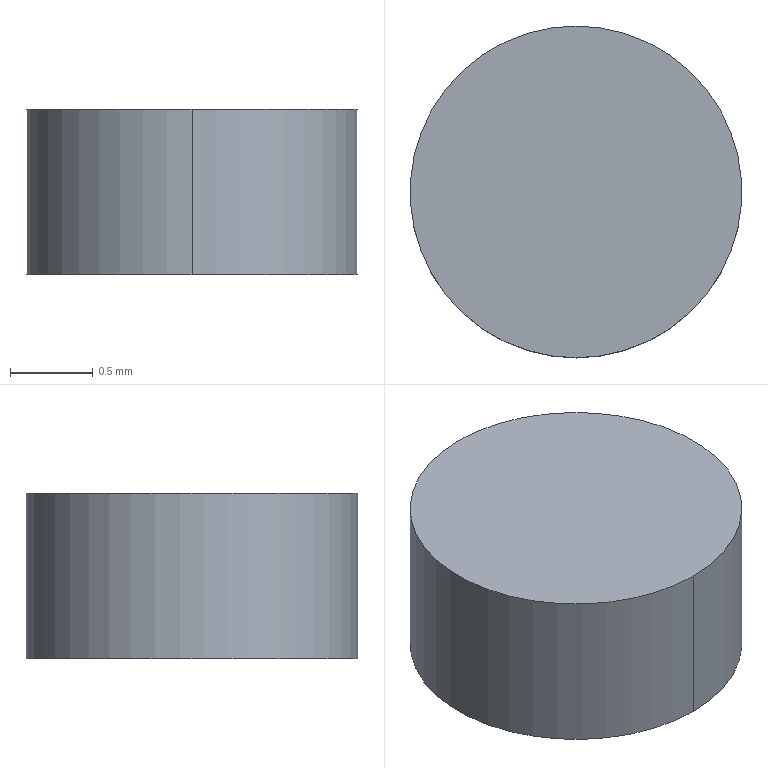Part | STEP file | 1 solid | 4 faces | box 2 x 2 x 1 mm | volume 3.142 mm3 | plane 2 | cylinder 2 | commonest cylinder face diameters 2 x2
STEP:
#1=CARTESIAN_POINT('',(0.,0.,0.));
#2=DIRECTION('',(0.,0.,1.));
#3=DIRECTION('',(1.,0.,0.));
#4=AXIS2_PLACEMENT_3D('',#1,#2,#3);
#5=CARTESIAN_POINT('',(-545.073,5728.073,1777.644));
#6=VERTEX_POINT('',#5);
#7=CARTESIAN_POINT('',(-545.073,5726.073,1777.644));
#8=VERTEX_POINT('',#7);
#9=CARTESIAN_POINT('',(-545.073,5727.073,1777.644));
#10=DIRECTION('',(0.,0.,-1.));
#11=DIRECTION('',(0.,1.,0.));
#12=AXIS2_PLACEMENT_3D('',#9,#10,#11);
#13=CIRCLE('',#12,1.);
#14=CARTESIAN_POINT('',(-529.573,5742.573,1777.644));
#15=DIRECTION('',(0.,0.,-1.));
#16=DIRECTION('',(-1.,0.,0.));
#17=AXIS2_PLACEMENT_3D('',#14,#15,#16);
#18=PLANE('',#17);
#19=CARTESIAN_POINT('',(15.5,-15.5));
#20=DIRECTION('',(0.,1.));
#21=AXIS2_PLACEMENT_2D('',#19,#20);
#22=CIRCLE('',#21,1.);
#23=(GEOMETRIC_REPRESENTATION_CONTEXT(2)PARAMETRIC_REPRESENTATION_CONTEXT()REPRESENTATION_CONTEXT('',''));
#24=DEFINITIONAL_REPRESENTATION('',(#22),#23);
#25=PCURVE('',#18,#24);
#26=CARTESIAN_POINT('',(-545.073,5727.073,1778.144));
#27=DIRECTION('',(0.,0.,1.));
#28=DIRECTION('',(0.,1.,0.));
#29=AXIS2_PLACEMENT_3D('',#26,#27,#28);
#30=CYLINDRICAL_SURFACE('',#29,1.);
#31=CARTESIAN_POINT('',(6.283,-0.5));
#32=DIRECTION('',(-1.,0.));
#33=VECTOR('',#32,1.);
#34=LINE('',#31,#33);
#35=(GEOMETRIC_REPRESENTATION_CONTEXT(2)PARAMETRIC_REPRESENTATION_CONTEXT()REPRESENTATION_CONTEXT('',''));
#36=DEFINITIONAL_REPRESENTATION('',(#34),#35);
#37=PCURVE('',#30,#36);
#38=SURFACE_CURVE('',#13,(#25,#37),.PCURVE_S1.);
#39=EDGE_CURVE('',#6,#8,#38,.T.);
#40=ORIENTED_EDGE('',*,*,#39,.F.);
#41=CARTESIAN_POINT('',(-545.073,5727.073,1777.644));
#42=DIRECTION('',(0.,0.,-1.));
#43=DIRECTION('',(0.,-1.,0.));
#44=AXIS2_PLACEMENT_3D('',#41,#42,#43);
#45=CIRCLE('',#44,1.);
#46=CARTESIAN_POINT('',(15.5,-15.5));
#47=DIRECTION('',(0.,-1.));
#48=AXIS2_PLACEMENT_2D('',#46,#47);
#49=CIRCLE('',#48,1.);
#50=(GEOMETRIC_REPRESENTATION_CONTEXT(2)PARAMETRIC_REPRESENTATION_CONTEXT()REPRESENTATION_CONTEXT('',''));
#51=DEFINITIONAL_REPRESENTATION('',(#49),#50);
#52=PCURVE('',#18,#51);
#53=CARTESIAN_POINT('',(-545.073,5727.073,1778.144));
#54=DIRECTION('',(0.,0.,1.));
#55=DIRECTION('',(0.,-1.,0.));
#56=AXIS2_PLACEMENT_3D('',#53,#54,#55);
#57=CYLINDRICAL_SURFACE('',#56,1.);
#58=CARTESIAN_POINT('',(6.283,-0.5));
#59=DIRECTION('',(-1.,0.));
#60=VECTOR('',#59,1.);
#61=LINE('',#58,#60);
#62=(GEOMETRIC_REPRESENTATION_CONTEXT(2)PARAMETRIC_REPRESENTATION_CONTEXT()REPRESENTATION_CONTEXT('',''));
#63=DEFINITIONAL_REPRESENTATION('',(#61),#62);
#64=PCURVE('',#57,#63);
#65=SURFACE_CURVE('',#45,(#52,#64),.PCURVE_S1.);
#66=EDGE_CURVE('',#8,#6,#65,.T.);
#67=ORIENTED_EDGE('',*,*,#66,.F.);
#68=EDGE_LOOP('',(#40,#67));
#69=FACE_BOUND('',#68,.F.);
#70=ADVANCED_FACE('',(#69),#18,.T.);
#71=CARTESIAN_POINT('',(-545.073,5726.073,1778.644));
#72=VERTEX_POINT('',#71);
#73=CARTESIAN_POINT('',(-545.073,5728.073,1778.644));
#74=VERTEX_POINT('',#73);
#75=CARTESIAN_POINT('',(-545.073,5727.073,1778.644));
#76=DIRECTION('',(0.,0.,1.));
#77=DIRECTION('',(0.,-1.,0.));
#78=AXIS2_PLACEMENT_3D('',#75,#76,#77);
#79=CIRCLE('',#78,1.);
#80=CARTESIAN_POINT('',(3.142,0.5));
#81=DIRECTION('',(1.,0.));
#82=VECTOR('',#81,1.);
#83=LINE('',#80,#82);
#84=(GEOMETRIC_REPRESENTATION_CONTEXT(2)PARAMETRIC_REPRESENTATION_CONTEXT()REPRESENTATION_CONTEXT('',''));
#85=DEFINITIONAL_REPRESENTATION('',(#83),#84);
#86=PCURVE('',#30,#85);
#87=CARTESIAN_POINT('',(-529.573,5742.573,1778.644));
#88=DIRECTION('',(0.,0.,-1.));
#89=DIRECTION('',(-1.,0.,0.));
#90=AXIS2_PLACEMENT_3D('',#87,#88,#89);
#91=PLANE('',#90);
#92=CARTESIAN_POINT('',(15.5,-16.5));
#93=CARTESIAN_POINT('',(13.768,-16.5));
#94=CARTESIAN_POINT('',(14.634,-15.));
#95=CARTESIAN_POINT('',(15.5,-13.5));
#96=CARTESIAN_POINT('',(16.366,-15.));
#97=CARTESIAN_POINT('',(17.232,-16.5));
#98=CARTESIAN_POINT('',(15.5,-16.5));
#99=(BOUNDED_CURVE()B_SPLINE_CURVE(2,(#92,#93,#94,#95,#96,#97,#98),.UNSPECIFIED.,.T.,.F.)B_SPLINE_CURVE_WITH_KNOTS((1,2,2,2,2,1),(-2.094,0.,2.094,4.189,6.283,8.378),.UNSPECIFIED.)CURVE()GEOMETRIC_REPRESENTATION_ITEM()RATIONAL_B_SPLINE_CURVE((1.,0.5,1.,0.5,1.,0.5,1.))REPRESENTATION_ITEM(''));
#100=(GEOMETRIC_REPRESENTATION_CONTEXT(2)PARAMETRIC_REPRESENTATION_CONTEXT()REPRESENTATION_CONTEXT('',''));
#101=DEFINITIONAL_REPRESENTATION('',(#99),#100);
#102=PCURVE('',#91,#101);
#103=SURFACE_CURVE('',#79,(#86,#102),.PCURVE_S1.);
#104=EDGE_CURVE('',#72,#74,#103,.T.);
#105=ORIENTED_EDGE('',*,*,#104,.F.);
#106=CARTESIAN_POINT('',(-545.073,5726.073,1778.644));
#107=DIRECTION('',(0.,0.,-1.));
#108=VECTOR('',#107,1.);
#109=LINE('',#106,#108);
#110=CARTESIAN_POINT('',(3.142,0.5));
#111=DIRECTION('',(0.,-1.));
#112=VECTOR('',#111,1.);
#113=LINE('',#110,#112);
#114=(GEOMETRIC_REPRESENTATION_CONTEXT(2)PARAMETRIC_REPRESENTATION_CONTEXT()REPRESENTATION_CONTEXT('',''));
#115=DEFINITIONAL_REPRESENTATION('',(#113),#114);
#116=PCURVE('',#30,#115);
#117=CARTESIAN_POINT('',(6.283,0.5));
#118=DIRECTION('',(0.,-1.));
#119=VECTOR('',#118,1.);
#120=LINE('',#117,#119);
#121=(GEOMETRIC_REPRESENTATION_CONTEXT(2)PARAMETRIC_REPRESENTATION_CONTEXT()REPRESENTATION_CONTEXT('',''));
#122=DEFINITIONAL_REPRESENTATION('',(#120),#121);
#123=PCURVE('',#57,#122);
#124=SURFACE_CURVE('',#109,(#116,#123),.PCURVE_S1.);
#125=EDGE_CURVE('',#72,#8,#124,.T.);
#126=ORIENTED_EDGE('',*,*,#125,.T.);
#127=ORIENTED_EDGE('',*,*,#39,.F.);
#128=CARTESIAN_POINT('',(-545.073,5728.073,1778.644));
#129=DIRECTION('',(0.,0.,-1.));
#130=VECTOR('',#129,1.);
#131=LINE('',#128,#130);
#132=CARTESIAN_POINT('',(6.283,0.5));
#133=DIRECTION('',(0.,-1.));
#134=VECTOR('',#133,1.);
#135=LINE('',#132,#134);
#136=(GEOMETRIC_REPRESENTATION_CONTEXT(2)PARAMETRIC_REPRESENTATION_CONTEXT()REPRESENTATION_CONTEXT('',''));
#137=DEFINITIONAL_REPRESENTATION('',(#135),#136);
#138=PCURVE('',#30,#137);
#139=CARTESIAN_POINT('',(3.142,0.5));
#140=DIRECTION('',(0.,-1.));
#141=VECTOR('',#140,1.);
#142=LINE('',#139,#141);
#143=(GEOMETRIC_REPRESENTATION_CONTEXT(2)PARAMETRIC_REPRESENTATION_CONTEXT()REPRESENTATION_CONTEXT('',''));
#144=DEFINITIONAL_REPRESENTATION('',(#142),#143);
#145=PCURVE('',#57,#144);
#146=SURFACE_CURVE('',#131,(#138,#145),.PCURVE_S1.);
#147=EDGE_CURVE('',#74,#6,#146,.T.);
#148=ORIENTED_EDGE('',*,*,#147,.F.);
#149=EDGE_LOOP('',(#105,#126,#127,#148));
#150=FACE_BOUND('',#149,.T.);
#151=ADVANCED_FACE('',(#150),#30,.T.);
#152=CARTESIAN_POINT('',(-545.073,5727.073,1778.644));
#153=DIRECTION('',(0.,0.,1.));
#154=DIRECTION('',(0.,1.,0.));
#155=AXIS2_PLACEMENT_3D('',#152,#153,#154);
#156=CIRCLE('',#155,1.);
#157=CARTESIAN_POINT('',(3.142,0.5));
#158=DIRECTION('',(1.,0.));
#159=VECTOR('',#158,1.);
#160=LINE('',#157,#159);
#161=(GEOMETRIC_REPRESENTATION_CONTEXT(2)PARAMETRIC_REPRESENTATION_CONTEXT()REPRESENTATION_CONTEXT('',''));
#162=DEFINITIONAL_REPRESENTATION('',(#160),#161);
#163=PCURVE('',#57,#162);
#164=CARTESIAN_POINT('',(15.5,-14.5));
#165=CARTESIAN_POINT('',(17.232,-14.5));
#166=CARTESIAN_POINT('',(16.366,-16.));
#167=CARTESIAN_POINT('',(15.5,-17.5));
#168=CARTESIAN_POINT('',(14.634,-16.));
#169=CARTESIAN_POINT('',(13.768,-14.5));
#170=CARTESIAN_POINT('',(15.5,-14.5));
#171=(BOUNDED_CURVE()B_SPLINE_CURVE(2,(#164,#165,#166,#167,#168,#169,#170),.UNSPECIFIED.,.T.,.F.)B_SPLINE_CURVE_WITH_KNOTS((1,2,2,2,2,1),(-2.094,0.,2.094,4.189,6.283,8.378),.UNSPECIFIED.)CURVE()GEOMETRIC_REPRESENTATION_ITEM()RATIONAL_B_SPLINE_CURVE((1.,0.5,1.,0.5,1.,0.5,1.))REPRESENTATION_ITEM(''));
#172=(GEOMETRIC_REPRESENTATION_CONTEXT(2)PARAMETRIC_REPRESENTATION_CONTEXT()REPRESENTATION_CONTEXT('',''));
#173=DEFINITIONAL_REPRESENTATION('',(#171),#172);
#174=PCURVE('',#91,#173);
#175=SURFACE_CURVE('',#156,(#163,#174),.PCURVE_S1.);
#176=EDGE_CURVE('',#74,#72,#175,.T.);
#177=ORIENTED_EDGE('',*,*,#176,.F.);
#178=ORIENTED_EDGE('',*,*,#147,.T.);
#179=ORIENTED_EDGE('',*,*,#66,.F.);
#180=ORIENTED_EDGE('',*,*,#125,.F.);
#181=EDGE_LOOP('',(#177,#178,#179,#180));
#182=FACE_BOUND('',#181,.T.);
#183=ADVANCED_FACE('',(#182),#57,.T.);
#184=ORIENTED_EDGE('',*,*,#104,.F.);
#185=ORIENTED_EDGE('',*,*,#176,.F.);
#186=EDGE_LOOP('',(#184,#185));
#187=FACE_BOUND('',#186,.F.);
#188=ADVANCED_FACE('',(#187),#91,.F.);
#189=CLOSED_SHELL('',(#70,#151,#183,#188));
#190=MANIFOLD_SOLID_BREP('',#189);
#191=(LENGTH_UNIT()NAMED_UNIT(*)SI_UNIT(.MILLI.,.METRE.));
#192=UNCERTAINTY_MEASURE_WITH_UNIT(LENGTH_MEASURE(0.0000001),#191,'','');
#193=(NAMED_UNIT(*)PLANE_ANGLE_UNIT()SI_UNIT($,.RADIAN.));
#194=(NAMED_UNIT(*)SI_UNIT($,.STERADIAN.)SOLID_ANGLE_UNIT());
#195=(GEOMETRIC_REPRESENTATION_CONTEXT(3)GLOBAL_UNCERTAINTY_ASSIGNED_CONTEXT((#192))GLOBAL_UNIT_ASSIGNED_CONTEXT((#191,#193,#194))REPRESENTATION_CONTEXT('',''));
#196=ADVANCED_BREP_SHAPE_REPRESENTATION('',(#4,#190),#195);